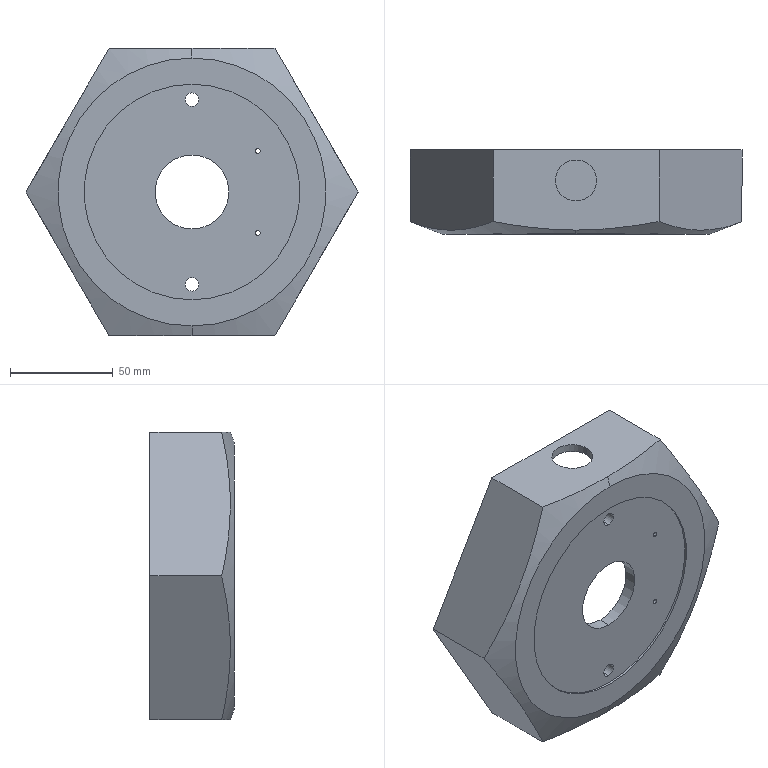Part | SolidWorks | features ICE 6, HoleWzd 2, Extrusion 1, RevCut 1 | 1 solid | 84 faces | box 161.658 x 41 x 140 mm | volume 170497 mm3 | plane 46 | cylinder 20 | cone 18 | commonest cylinder face diameters 2.5 x10 6.5 x4 20 x2 36 x2 105 x2